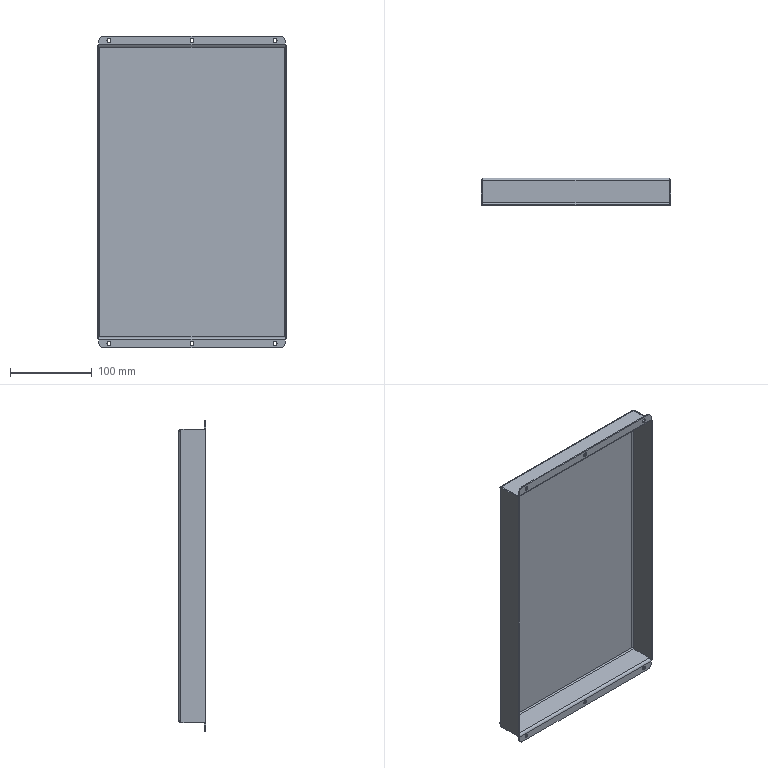Part | NX | features BREP 1 | 1 solid | 82 faces | box 231.597 x 33.249 x 381 mm | volume 185305 mm3 | plane 54 | cylinder 28 | commonest cylinder face diameters 4.826 x12 3.175 x6 6.172 x6 12.7 x4